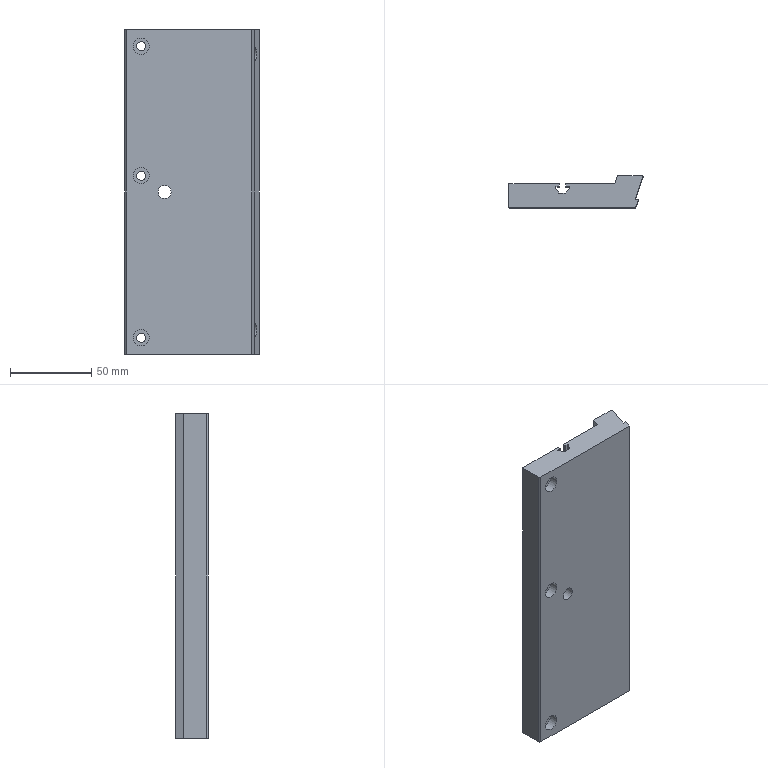Part | STEP file | 1 solid | 42 faces | box 82.749 x 20 x 200 mm | volume 243031 mm3 | plane 21 | cylinder 19 | cone 2 | commonest cylinder face diameters 1 x9 5.5 x3 8 x3 10 x3 2 x1